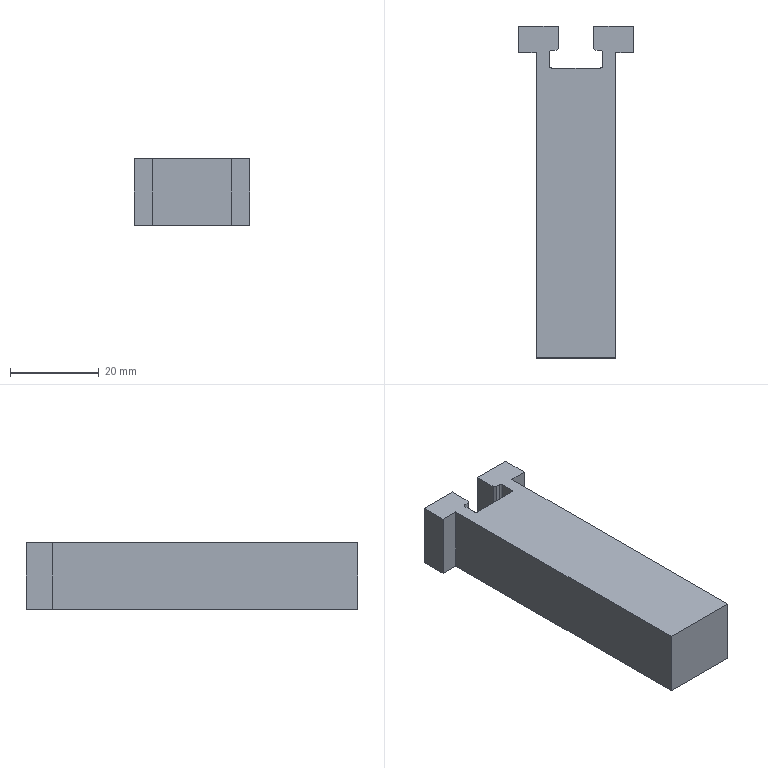Part | STEP file | PN_0052 | 1 solid | 24 faces | box 26 x 75 x 15 mm | volume 19589 mm3 | plane 20 | cylinder 4 | commonest cylinder face diameters 1 x4